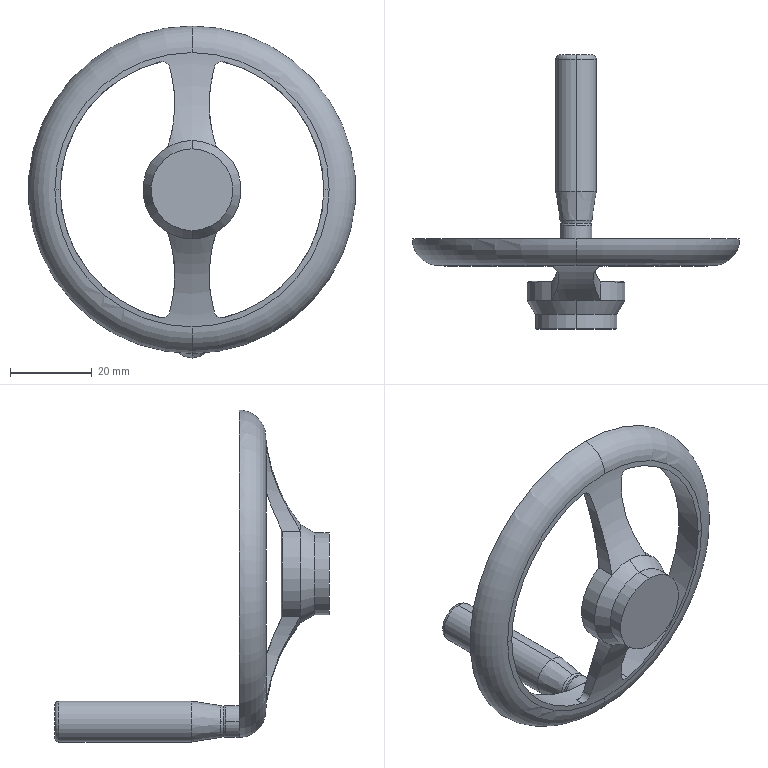Part | STEP file | fSHLN80 | 1 solid | 44 faces | box 80 x 67 x 81.1 mm | volume 18367 mm3 | cylinder 20 | cone 10 | other 6 | torus 4 | plane 4 | commonest cylinder face diameters 4 x6 64 x4 7.8 x2 10 x2 20 x2 24 x2